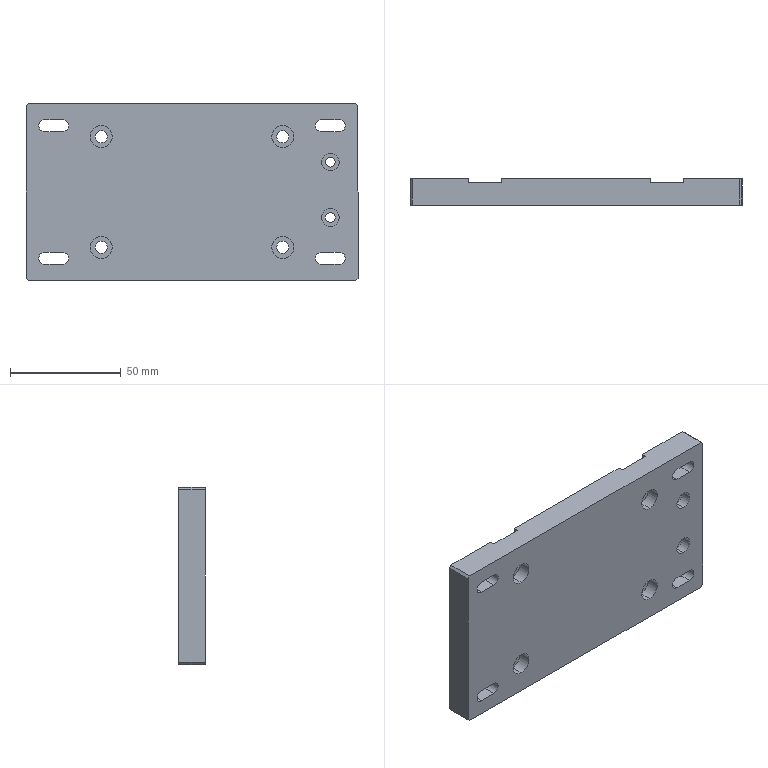Part | SolidWorks | features HoleWzd 3, Chamfer 1, Extrusion 1, ICE 1 | 1 solid | 84 faces | box 150 x 12 x 80 mm | volume 130957 mm3 | plane 44 | cylinder 40 | commonest cylinder face diameters 5.5 x16 10 x16 4.5 x4 8 x4